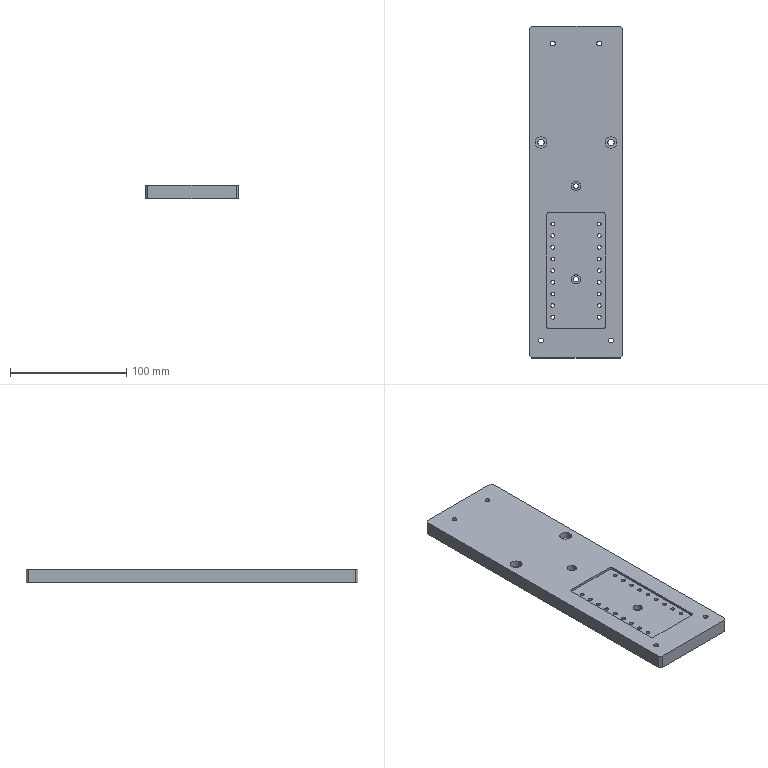Part | SolidWorks | features HoleWzd 5, Chamfer 1, Extrusion 1, ICE 1 | 1 solid | 83 faces | box 80 x 285 x 12 mm | volume 259377 mm3 | cylinder 64 | plane 19 | commonest cylinder face diameters 3.3 x36 4.2 x8 4 x4 4.5 x4 5.5 x4 8 x4